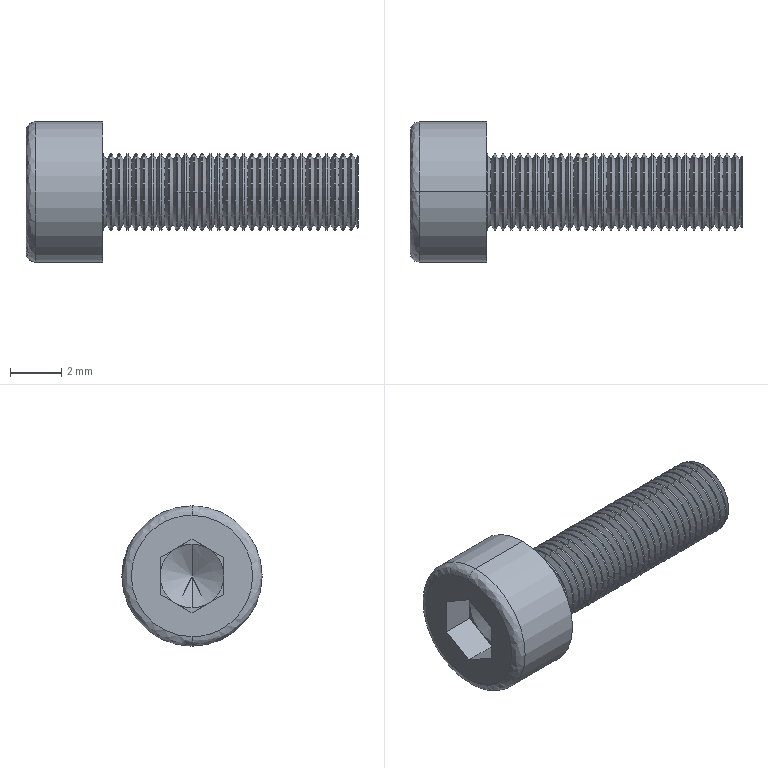Part | SolidWorks | features BaseBody 1 | 1 solid | 209 faces | box 13 x 5.5 x 5.5 mm | volume 124.477 mm3 | cone 128 | cylinder 64 | plane 15 | spline 2 | commonest cylinder face diameters 3 x62 5.5 x2